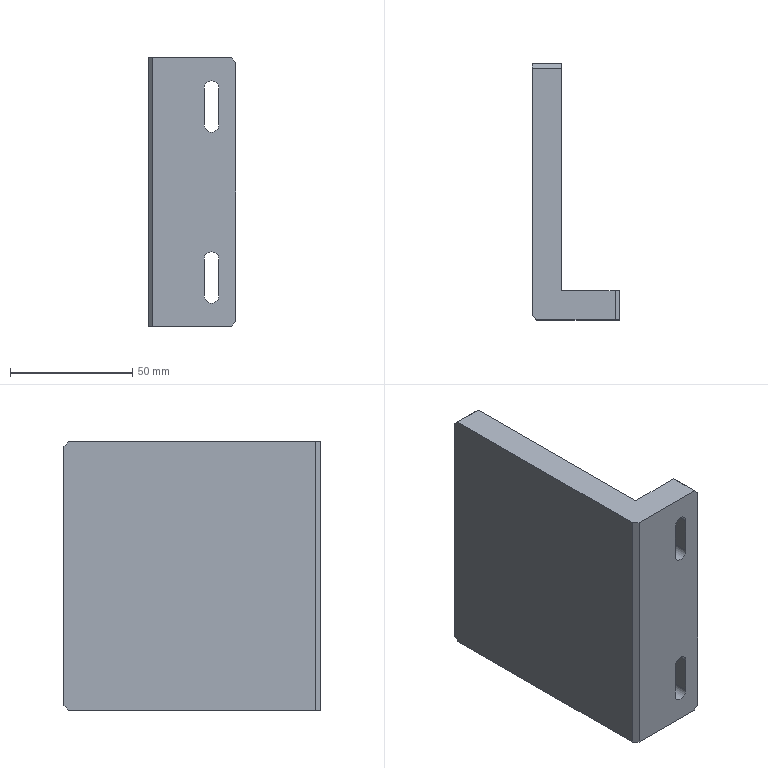Part | SolidWorks | features Chamfer 1, Extrusion 1, HoleWzd 1, ICE 1 | 1 solid | 31 faces | box 36 x 105 x 110 mm | volume 166694 mm3 | plane 17 | cylinder 10 | cone 4 | commonest cylinder face diameters 6 x6 5 x4
STEP:
#1=CARTESIAN_POINT('',(-32.601,41.28,96.5));
#2=VERTEX_POINT('',#1);
#3=CARTESIAN_POINT('',(-32.601,41.28,101.5));
#4=VERTEX_POINT('',#3);
#5=CARTESIAN_POINT('',(-32.601,41.28,99.));
#6=DIRECTION('',(0.,1.,0.));
#7=DIRECTION('',(0.,0.,1.));
#8=AXIS2_PLACEMENT_3D('',#5,#6,#7);
#9=CIRCLE('',#8,2.5);
#10=EDGE_CURVE('',#2,#4,#9,.T.);
#11=ORIENTED_EDGE('',*,*,#10,.F.);
#12=CARTESIAN_POINT('',(-32.601,51.778,96.5));
#13=VERTEX_POINT('',#12);
#14=CARTESIAN_POINT('',(-32.601,51.778,96.5));
#15=DIRECTION('',(0.,1.,0.));
#16=VECTOR('',#15,1000.);
#17=LINE('',#14,#16);
#18=EDGE_CURVE('',#2,#13,#17,.T.);
#19=ORIENTED_EDGE('',*,*,#18,.T.);
#20=CARTESIAN_POINT('',(-32.601,51.778,101.5));
#21=VERTEX_POINT('',#20);
#22=CARTESIAN_POINT('',(-32.601,51.778,99.));
#23=DIRECTION('',(0.,1.,0.));
#24=DIRECTION('',(0.,0.,1.));
#25=AXIS2_PLACEMENT_3D('',#22,#23,#24);
#26=CIRCLE('',#25,2.5);
#27=EDGE_CURVE('',#13,#21,#26,.T.);
#28=ORIENTED_EDGE('',*,*,#27,.T.);
#29=CARTESIAN_POINT('',(-32.601,51.778,101.5));
#30=DIRECTION('',(0.,1.,0.));
#31=VECTOR('',#30,1000.);
#32=LINE('',#29,#31);
#33=EDGE_CURVE('',#4,#21,#32,.T.);
#34=ORIENTED_EDGE('',*,*,#33,.F.);
#35=EDGE_LOOP('',(#11,#19,#28,#34));
#36=FACE_OUTER_BOUND('',#35,.T.);
#37=CARTESIAN_POINT('',(-32.601,51.778,99.));
#38=DIRECTION('',(0.,1.,0.));
#39=DIRECTION('',(0.,0.,1.));
#40=AXIS2_PLACEMENT_3D('',#37,#38,#39);
#41=CYLINDRICAL_SURFACE('',#40,2.5);
#42=ADVANCED_FACE('',(#36),#41,.F.);
#43=CARTESIAN_POINT('',(-32.601,39.778,99.));
#44=VERTEX_POINT('',#43);
#45=CARTESIAN_POINT('',(-32.601,41.28,101.5));
#46=DIRECTION('',(0.,0.515,0.8572));
#47=VECTOR('',#46,1000.);
#48=LINE('',#45,#47);
#49=EDGE_CURVE('',#44,#4,#48,.T.);
#50=ORIENTED_EDGE('',*,*,#49,.F.);
#51=CARTESIAN_POINT('',(-32.601,41.28,96.5));
#52=DIRECTION('',(0.,0.515,-0.8572));
#53=VECTOR('',#52,1000.);
#54=LINE('',#51,#53);
#55=EDGE_CURVE('',#44,#2,#54,.T.);
#56=ORIENTED_EDGE('',*,*,#55,.T.);
#57=ORIENTED_EDGE('',*,*,#10,.T.);
#58=EDGE_LOOP('',(#50,#56,#57));
#59=FACE_OUTER_BOUND('',#58,.T.);
#60=CARTESIAN_POINT('',(-32.601,41.28,99.));
#61=DIRECTION('',(0.,1.,0.));
#62=DIRECTION('',(0.,0.,1.));
#63=AXIS2_PLACEMENT_3D('',#60,#61,#62);
#64=CONICAL_SURFACE('',#63,2.5,1.03);
#65=ADVANCED_FACE('',(#59),#64,.F.);
#66=CARTESIAN_POINT('',(-32.601,41.28,8.5));
#67=VERTEX_POINT('',#66);
#68=CARTESIAN_POINT('',(-32.601,41.28,13.5));
#69=VERTEX_POINT('',#68);
#70=CARTESIAN_POINT('',(-32.601,41.28,11.));
#71=DIRECTION('',(0.,1.,0.));
#72=DIRECTION('',(0.,0.,1.));
#73=AXIS2_PLACEMENT_3D('',#70,#71,#72);
#74=CIRCLE('',#73,2.5);
#75=EDGE_CURVE('',#67,#69,#74,.T.);
#76=ORIENTED_EDGE('',*,*,#75,.F.);
#77=CARTESIAN_POINT('',(-32.601,51.778,8.5));
#78=VERTEX_POINT('',#77);
#79=CARTESIAN_POINT('',(-32.601,51.778,8.5));
#80=DIRECTION('',(0.,1.,0.));
#81=VECTOR('',#80,1000.);
#82=LINE('',#79,#81);
#83=EDGE_CURVE('',#67,#78,#82,.T.);
#84=ORIENTED_EDGE('',*,*,#83,.T.);
#85=CARTESIAN_POINT('',(-32.601,51.778,13.5));
#86=VERTEX_POINT('',#85);
#87=CARTESIAN_POINT('',(-32.601,51.778,11.));
#88=DIRECTION('',(0.,1.,0.));
#89=DIRECTION('',(0.,0.,1.));
#90=AXIS2_PLACEMENT_3D('',#87,#88,#89);
#91=CIRCLE('',#90,2.5);
#92=EDGE_CURVE('',#78,#86,#91,.T.);
#93=ORIENTED_EDGE('',*,*,#92,.T.);
#94=CARTESIAN_POINT('',(-32.601,51.778,13.5));
#95=DIRECTION('',(0.,1.,0.));
#96=VECTOR('',#95,1000.);
#97=LINE('',#94,#96);
#98=EDGE_CURVE('',#69,#86,#97,.T.);
#99=ORIENTED_EDGE('',*,*,#98,.F.);
#100=EDGE_LOOP('',(#76,#84,#93,#99));
#101=FACE_OUTER_BOUND('',#100,.T.);
#102=CARTESIAN_POINT('',(-32.601,51.778,11.));
#103=DIRECTION('',(0.,1.,0.));
#104=DIRECTION('',(0.,0.,1.));
#105=AXIS2_PLACEMENT_3D('',#102,#103,#104);
#106=CYLINDRICAL_SURFACE('',#105,2.5);
#107=ADVANCED_FACE('',(#101),#106,.F.);
#108=CARTESIAN_POINT('',(-32.601,39.778,11.));
#109=VERTEX_POINT('',#108);
#110=CARTESIAN_POINT('',(-32.601,41.28,13.5));
#111=DIRECTION('',(0.,0.515,0.8572));
#112=VECTOR('',#111,1000.);
#113=LINE('',#110,#112);
#114=EDGE_CURVE('',#109,#69,#113,.T.);
#115=ORIENTED_EDGE('',*,*,#114,.F.);
#116=CARTESIAN_POINT('',(-32.601,41.28,8.5));
#117=DIRECTION('',(0.,0.515,-0.8572));
#118=VECTOR('',#117,1000.);
#119=LINE('',#116,#118);
#120=EDGE_CURVE('',#109,#67,#119,.T.);
#121=ORIENTED_EDGE('',*,*,#120,.T.);
#122=ORIENTED_EDGE('',*,*,#75,.T.);
#123=EDGE_LOOP('',(#115,#121,#122));
#124=FACE_OUTER_BOUND('',#123,.T.);
#125=CARTESIAN_POINT('',(-32.601,41.28,11.));
#126=DIRECTION('',(0.,1.,0.));
#127=DIRECTION('',(0.,0.,1.));
#128=AXIS2_PLACEMENT_3D('',#125,#126,#127);
#129=CONICAL_SURFACE('',#128,2.5,1.03);
#130=ADVANCED_FACE('',(#124),#129,.F.);
#131=CARTESIAN_POINT('',(-12.601,-53.222,100.5));
#132=VERTEX_POINT('',#131);
#133=CARTESIAN_POINT('',(-9.601,-53.222,97.5));
#134=VERTEX_POINT('',#133);
#135=CARTESIAN_POINT('',(-12.601,-53.222,97.5));
#136=DIRECTION('',(0.,1.,0.));
#137=DIRECTION('',(0.,0.,1.));
#138=AXIS2_PLACEMENT_3D('',#135,#136,#137);
#139=CIRCLE('',#138,3.);
#140=EDGE_CURVE('',#132,#134,#139,.T.);
#141=ORIENTED_EDGE('',*,*,#140,.F.);
#142=CARTESIAN_POINT('',(-12.601,-41.222,100.5));
#143=VERTEX_POINT('',#142);
#144=CARTESIAN_POINT('',(-12.601,-53.222,100.5));
#145=DIRECTION('',(0.,1.,0.));
#146=VECTOR('',#145,1000.);
#147=LINE('',#144,#146);
#148=EDGE_CURVE('',#132,#143,#147,.T.);
#149=ORIENTED_EDGE('',*,*,#148,.T.);
#150=CARTESIAN_POINT('',(-9.601,-41.222,97.5));
#151=VERTEX_POINT('',#150);
#152=CARTESIAN_POINT('',(-12.601,-41.222,97.5));
#153=DIRECTION('',(0.,1.,0.));
#154=DIRECTION('',(0.,0.,1.));
#155=AXIS2_PLACEMENT_3D('',#152,#153,#154);
#156=CIRCLE('',#155,3.);
#157=EDGE_CURVE('',#143,#151,#156,.T.);
#158=ORIENTED_EDGE('',*,*,#157,.T.);
#159=CARTESIAN_POINT('',(-9.601,-53.222,97.5));
#160=DIRECTION('',(0.,1.,0.));
#161=VECTOR('',#160,1000.);
#162=LINE('',#159,#161);
#163=EDGE_CURVE('',#134,#151,#162,.T.);
#164=ORIENTED_EDGE('',*,*,#163,.F.);
#165=EDGE_LOOP('',(#141,#149,#158,#164));
#166=FACE_OUTER_BOUND('',#165,.T.);
#167=CARTESIAN_POINT('',(-12.601,-53.222,97.5));
#168=DIRECTION('',(0.,1.,0.));
#169=DIRECTION('',(0.,0.,1.));
#170=AXIS2_PLACEMENT_3D('',#167,#168,#169);
#171=CYLINDRICAL_SURFACE('',#170,3.);
#172=ADVANCED_FACE('',(#166),#171,.F.);
#173=CARTESIAN_POINT('',(-12.601,-53.222,30.5));
#174=VERTEX_POINT('',#173);
#175=CARTESIAN_POINT('',(-9.601,-53.222,27.5));
#176=VERTEX_POINT('',#175);
#177=CARTESIAN_POINT('',(-12.601,-53.222,27.5));
#178=DIRECTION('',(0.,1.,0.));
#179=DIRECTION('',(0.,0.,-1.));
#180=AXIS2_PLACEMENT_3D('',#177,#178,#179);
#181=CIRCLE('',#180,3.);
#182=EDGE_CURVE('',#174,#176,#181,.T.);
#183=ORIENTED_EDGE('',*,*,#182,.F.);
#184=CARTESIAN_POINT('',(-12.601,-41.222,30.5));
#185=VERTEX_POINT('',#184);
#186=CARTESIAN_POINT('',(-12.601,-53.222,30.5));
#187=DIRECTION('',(0.,1.,0.));
#188=VECTOR('',#187,1000.);
#189=LINE('',#186,#188);
#190=EDGE_CURVE('',#174,#185,#189,.T.);
#191=ORIENTED_EDGE('',*,*,#190,.T.);
#192=CARTESIAN_POINT('',(-9.601,-41.222,27.5));
#193=VERTEX_POINT('',#192);
#194=CARTESIAN_POINT('',(-12.601,-41.222,27.5));
#195=DIRECTION('',(0.,1.,0.));
#196=DIRECTION('',(0.,0.,-1.));
#197=AXIS2_PLACEMENT_3D('',#194,#195,#196);
#198=CIRCLE('',#197,3.);
#199=EDGE_CURVE('',#185,#193,#198,.T.);
#200=ORIENTED_EDGE('',*,*,#199,.T.);
#201=CARTESIAN_POINT('',(-9.601,-53.222,27.5));
#202=DIRECTION('',(0.,1.,0.));
#203=VECTOR('',#202,1000.);
#204=LINE('',#201,#203);
#205=EDGE_CURVE('',#176,#193,#204,.T.);
#206=ORIENTED_EDGE('',*,*,#205,.F.);
#207=EDGE_LOOP('',(#183,#191,#200,#206));
#208=FACE_OUTER_BOUND('',#207,.T.);
#209=CARTESIAN_POINT('',(-12.601,-53.222,27.5));
#210=DIRECTION('',(0.,1.,0.));
#211=DIRECTION('',(0.,0.,1.));
#212=AXIS2_PLACEMENT_3D('',#209,#210,#211);
#213=CYLINDRICAL_SURFACE('',#212,3.);
#214=ADVANCED_FACE('',(#208),#213,.F.);
#215=CARTESIAN_POINT('',(-32.601,51.778,99.));
#216=DIRECTION('',(0.,1.,0.));
#217=DIRECTION('',(0.,0.,1.));
#218=AXIS2_PLACEMENT_3D('',#215,#216,#217);
#219=CIRCLE('',#218,2.5);
#220=EDGE_CURVE('',#21,#13,#219,.T.);
#221=ORIENTED_EDGE('',*,*,#220,.F.);
#222=ORIENTED_EDGE('',*,*,#27,.F.);
#223=EDGE_LOOP('',(#221,#222));
#224=FACE_BOUND('',#223,.T.);
#225=CARTESIAN_POINT('',(-32.601,51.778,11.));
#226=DIRECTION('',(0.,1.,0.));
#227=DIRECTION('',(0.,0.,1.));
#228=AXIS2_PLACEMENT_3D('',#225,#226,#227);
#229=CIRCLE('',#228,2.5);
#230=EDGE_CURVE('',#86,#78,#229,.T.);
#231=ORIENTED_EDGE('',*,*,#230,.F.);
#232=ORIENTED_EDGE('',*,*,#92,.F.);
#233=EDGE_LOOP('',(#231,#232));
#234=FACE_BOUND('',#233,.T.);
#235=CARTESIAN_POINT('',(-26.601,51.778,108.));
#236=VERTEX_POINT('',#235);
#237=CARTESIAN_POINT('',(-26.601,51.778,2.));
#238=VERTEX_POINT('',#237);
#239=CARTESIAN_POINT('',(-26.601,51.778,110.));
#240=DIRECTION('',(0.,0.,-1.));
#241=VECTOR('',#240,1000.);
#242=LINE('',#239,#241);
#243=EDGE_CURVE('',#236,#238,#242,.T.);
#244=ORIENTED_EDGE('',*,*,#243,.T.);
#245=CARTESIAN_POINT('',(-38.601,51.778,2.));
#246=VERTEX_POINT('',#245);
#247=CARTESIAN_POINT('',(-26.601,51.778,2.));
#248=DIRECTION('',(-1.,0.,0.));
#249=VECTOR('',#248,1000.);
#250=LINE('',#247,#249);
#251=EDGE_CURVE('',#238,#246,#250,.T.);
#252=ORIENTED_EDGE('',*,*,#251,.T.);
#253=CARTESIAN_POINT('',(-38.601,51.778,108.));
#254=VERTEX_POINT('',#253);
#255=CARTESIAN_POINT('',(-38.601,51.778,110.));
#256=DIRECTION('',(0.,0.,-1.));
#257=VECTOR('',#256,1000.);
#258=LINE('',#255,#257);
#259=EDGE_CURVE('',#254,#246,#258,.T.);
#260=ORIENTED_EDGE('',*,*,#259,.F.);
#261=CARTESIAN_POINT('',(-26.601,51.778,108.));
#262=DIRECTION('',(1.,0.,0.));
#263=VECTOR('',#262,1000.);
#264=LINE('',#261,#263);
#265=EDGE_CURVE('',#254,#236,#264,.T.);
#266=ORIENTED_EDGE('',*,*,#265,.T.);
#267=EDGE_LOOP('',(#244,#252,#260,#266));
#268=FACE_OUTER_BOUND('',#267,.T.);
#269=CARTESIAN_POINT('',(-26.601,51.778,110.));
#270=DIRECTION('',(0.,-1.,0.));
#271=DIRECTION('',(1.,0.,0.));
#272=AXIS2_PLACEMENT_3D('',#269,#270,#271);
#273=PLANE('',#272);
#274=ADVANCED_FACE('',(#224,#234,#268),#273,.F.);
#275=CARTESIAN_POINT('',(-38.601,49.778,0.));
#276=VERTEX_POINT('',#275);
#277=CARTESIAN_POINT('',(-38.601,-51.222,0.));
#278=VERTEX_POINT('',#277);
#279=CARTESIAN_POINT('',(-38.601,51.778,0.));
#280=DIRECTION('',(0.,-1.,0.));
#281=VECTOR('',#280,1000.);
#282=LINE('',#279,#281);
#283=EDGE_CURVE('',#276,#278,#282,.T.);
#284=ORIENTED_EDGE('',*,*,#283,.T.);
#285=CARTESIAN_POINT('',(-38.601,-51.222,110.));
#286=VERTEX_POINT('',#285);
#287=CARTESIAN_POINT('',(-38.601,-51.222,110.));
#288=DIRECTION('',(0.,0.,1.));
#289=VECTOR('',#288,1000.);
#290=LINE('',#287,#289);
#291=EDGE_CURVE('',#278,#286,#290,.T.);
#292=ORIENTED_EDGE('',*,*,#291,.T.);
#293=CARTESIAN_POINT('',(-38.601,49.778,110.));
#294=VERTEX_POINT('',#293);
#295=CARTESIAN_POINT('',(-38.601,51.778,110.));
#296=DIRECTION('',(0.,-1.,0.));
#297=VECTOR('',#296,1000.);
#298=LINE('',#295,#297);
#299=EDGE_CURVE('',#294,#286,#298,.T.);
#300=ORIENTED_EDGE('',*,*,#299,.F.);
#301=CARTESIAN_POINT('',(-38.601,49.778,110.));
#302=DIRECTION('',(0.,0.7071,-0.7071));
#303=VECTOR('',#302,1000.);
#304=LINE('',#301,#303);
#305=EDGE_CURVE('',#294,#254,#304,.T.);
#306=ORIENTED_EDGE('',*,*,#305,.T.);
#307=ORIENTED_EDGE('',*,*,#259,.T.);
#308=CARTESIAN_POINT('',(-38.601,51.778,2.));
#309=DIRECTION('',(0.,-0.7071,-0.7071));
#310=VECTOR('',#309,1000.);
#311=LINE('',#308,#310);
#312=EDGE_CURVE('',#246,#276,#311,.T.);
#313=ORIENTED_EDGE('',*,*,#312,.T.);
#314=EDGE_LOOP('',(#284,#292,#300,#306,#307,#313));
#315=FACE_OUTER_BOUND('',#314,.T.);
#316=CARTESIAN_POINT('',(-38.601,51.778,110.));
#317=DIRECTION('',(1.,0.,0.));
#318=DIRECTION('',(0.,1.,0.));
#319=AXIS2_PLACEMENT_3D('',#316,#317,#318);
#320=PLANE('',#319);
#321=ADVANCED_FACE('',(#315),#320,.F.);
#322=CARTESIAN_POINT('',(-15.601,-53.222,82.5));
#323=VERTEX_POINT('',#322);
#324=CARTESIAN_POINT('',(-15.601,-53.222,97.5));
#325=VERTEX_POINT('',#324);
#326=CARTESIAN_POINT('',(-15.601,-53.222,97.5));
#327=DIRECTION('',(0.,0.,1.));
#328=VECTOR('',#327,1000.);
#329=LINE('',#326,#328);
#330=EDGE_CURVE('',#323,#325,#329,.T.);
#331=ORIENTED_EDGE('',*,*,#330,.T.);
#332=CARTESIAN_POINT('',(-12.601,-53.222,97.5));
#333=DIRECTION('',(0.,1.,0.));
#334=DIRECTION('',(0.,0.,1.));
#335=AXIS2_PLACEMENT_3D('',#332,#333,#334);
#336=CIRCLE('',#335,3.);
#337=EDGE_CURVE('',#325,#132,#336,.T.);
#338=ORIENTED_EDGE('',*,*,#337,.T.);
#339=ORIENTED_EDGE('',*,*,#140,.T.);
#340=CARTESIAN_POINT('',(-9.601,-53.222,82.5));
#341=VERTEX_POINT('',#340);
#342=CARTESIAN_POINT('',(-9.601,-53.222,97.5));
#343=DIRECTION('',(0.,0.,-1.));
#344=VECTOR('',#343,1000.);
#345=LINE('',#342,#344);
#346=EDGE_CURVE('',#134,#341,#345,.T.);
#347=ORIENTED_EDGE('',*,*,#346,.T.);
#348=CARTESIAN_POINT('',(-12.601,-53.222,82.5));
#349=DIRECTION('',(0.,1.,0.));
#350=DIRECTION('',(0.,0.,1.));
#351=AXIS2_PLACEMENT_3D('',#348,#349,#350);
#352=CIRCLE('',#351,3.);
#353=EDGE_CURVE('',#341,#323,#352,.T.);
#354=ORIENTED_EDGE('',*,*,#353,.T.);
#355=EDGE_LOOP('',(#331,#338,#339,#347,#354));
#356=FACE_BOUND('',#355,.T.);
#357=CARTESIAN_POINT('',(-9.601,-53.222,12.5));
#358=VERTEX_POINT('',#357);
#359=CARTESIAN_POINT('',(-9.601,-53.222,12.5));
#360=DIRECTION('',(0.,0.,-1.));
#361=VECTOR('',#360,1000.);
#362=LINE('',#359,#361);
#363=EDGE_CURVE('',#176,#358,#362,.T.);
#364=ORIENTED_EDGE('',*,*,#363,.T.);
#365=CARTESIAN_POINT('',(-15.601,-53.222,12.5));
#366=VERTEX_POINT('',#365);
#367=CARTESIAN_POINT('',(-12.601,-53.222,12.5));
#368=DIRECTION('',(0.,1.,0.));
#369=DIRECTION('',(0.,0.,-1.));
#370=AXIS2_PLACEMENT_3D('',#367,#368,#369);
#371=CIRCLE('',#370,3.);
#372=EDGE_CURVE('',#358,#366,#371,.T.);
#373=ORIENTED_EDGE('',*,*,#372,.T.);
#374=CARTESIAN_POINT('',(-15.601,-53.222,27.5));
#375=VERTEX_POINT('',#374);
#376=CARTESIAN_POINT('',(-15.601,-53.222,12.5));
#377=DIRECTION('',(0.,0.,1.));
#378=VECTOR('',#377,1000.);
#379=LINE('',#376,#378);
#380=EDGE_CURVE('',#366,#375,#379,.T.);
#381=ORIENTED_EDGE('',*,*,#380,.T.);
#382=CARTESIAN_POINT('',(-12.601,-53.222,27.5));
#383=DIRECTION('',(0.,1.,0.));
#384=DIRECTION('',(0.,0.,-1.));
#385=AXIS2_PLACEMENT_3D('',#382,#383,#384);
#386=CIRCLE('',#385,3.);
#387=EDGE_CURVE('',#375,#174,#386,.T.);
#388=ORIENTED_EDGE('',*,*,#387,.T.);
#389=ORIENTED_EDGE('',*,*,#182,.T.);
#390=EDGE_LOOP('',(#364,#373,#381,#388,#389));
#391=FACE_BOUND('',#390,.T.);
#392=CARTESIAN_POINT('',(-36.601,-53.222,110.));
#393=VERTEX_POINT('',#392);
#394=CARTESIAN_POINT('',(-4.601,-53.222,110.));
#395=VERTEX_POINT('',#394);
#396=CARTESIAN_POINT('',(-38.601,-53.222,110.));
#397=DIRECTION('',(1.,0.,0.));
#398=VECTOR('',#397,1000.);
#399=LINE('',#396,#398);
#400=EDGE_CURVE('',#393,#395,#399,.T.);
#401=ORIENTED_EDGE('',*,*,#400,.F.);
#402=CARTESIAN_POINT('',(-36.601,-53.222,0.));
#403=VERTEX_POINT('',#402);
#404=CARTESIAN_POINT('',(-36.601,-53.222,110.));
#405=DIRECTION('',(0.,0.,-1.));
#406=VECTOR('',#405,1000.);
#407=LINE('',#404,#406);
#408=EDGE_CURVE('',#393,#403,#407,.T.);
#409=ORIENTED_EDGE('',*,*,#408,.T.);
#410=CARTESIAN_POINT('',(-4.601,-53.222,0.));
#411=VERTEX_POINT('',#410);
#412=CARTESIAN_POINT('',(-38.601,-53.222,0.));
#413=DIRECTION('',(1.,0.,0.));
#414=VECTOR('',#413,1000.);
#415=LINE('',#412,#414);
#416=EDGE_CURVE('',#403,#411,#415,.T.);
#417=ORIENTED_EDGE('',*,*,#416,.T.);
#418=CARTESIAN_POINT('',(-2.601,-53.222,2.));
#419=VERTEX_POINT('',#418);
#420=CARTESIAN_POINT('',(-2.601,-53.222,2.));
#421=DIRECTION('',(0.7071,0.,0.7071));
#422=VECTOR('',#421,1000.);
#423=LINE('',#420,#422);
#424=EDGE_CURVE('',#411,#419,#423,.T.);
#425=ORIENTED_EDGE('',*,*,#424,.T.);
#426=CARTESIAN_POINT('',(-2.601,-53.222,108.));
#427=VERTEX_POINT('',#426);
#428=CARTESIAN_POINT('',(-2.601,-53.222,110.));
#429=DIRECTION('',(0.,0.,-1.));
#430=VECTOR('',#429,1000.);
#431=LINE('',#428,#430);
#432=EDGE_CURVE('',#427,#419,#431,.T.);
#433=ORIENTED_EDGE('',*,*,#432,.F.);
#434=CARTESIAN_POINT('',(-4.601,-53.222,110.));
#435=DIRECTION('',(-0.7071,0.,0.7071));
#436=VECTOR('',#435,1000.);
#437=LINE('',#434,#436);
#438=EDGE_CURVE('',#427,#395,#437,.T.);
#439=ORIENTED_EDGE('',*,*,#438,.T.);
#440=EDGE_LOOP('',(#401,#409,#417,#425,#433,#439));
#441=FACE_OUTER_BOUND('',#440,.T.);
#442=CARTESIAN_POINT('',(-38.601,-53.222,110.));
#443=DIRECTION('',(0.,1.,0.));
#444=DIRECTION('',(0.,0.,1.));
#445=AXIS2_PLACEMENT_3D('',#442,#443,#444);
#446=PLANE('',#445);
#447=ADVANCED_FACE('',(#356,#391,#441),#446,.F.);
#448=ORIENTED_EDGE('',*,*,#432,.T.);
#449=CARTESIAN_POINT('',(-2.601,-41.222,2.));
#450=VERTEX_POINT('',#449);
#451=CARTESIAN_POINT('',(-2.601,-53.222,2.));
#452=DIRECTION('',(0.,1.,0.));
#453=VECTOR('',#452,1000.);
#454=LINE('',#451,#453);
#455=EDGE_CURVE('',#419,#450,#454,.T.);
#456=ORIENTED_EDGE('',*,*,#455,.T.);
#457=CARTESIAN_POINT('',(-2.601,-41.222,108.));
#458=VERTEX_POINT('',#457);
#459=CARTESIAN_POINT('',(-2.601,-41.222,110.));
#460=DIRECTION('',(0.,0.,-1.));
#461=VECTOR('',#460,1000.);
#462=LINE('',#459,#461);
#463=EDGE_CURVE('',#458,#450,#462,.T.);
#464=ORIENTED_EDGE('',*,*,#463,.F.);
#465=CARTESIAN_POINT('',(-2.601,-53.222,108.));
#466=DIRECTION('',(0.,-1.,0.));
#467=VECTOR('',#466,1000.);
#468=LINE('',#465,#467);
#469=EDGE_CURVE('',#458,#427,#468,.T.);
#470=ORIENTED_EDGE('',*,*,#469,.T.);
#471=EDGE_LOOP('',(#448,#456,#464,#470));
#472=FACE_OUTER_BOUND('',#471,.T.);
#473=CARTESIAN_POINT('',(-2.601,-53.222,110.));
#474=DIRECTION('',(-1.,0.,0.));
#475=DIRECTION('',(0.,0.,1.));
#476=AXIS2_PLACEMENT_3D('',#473,#474,#475);
#477=PLANE('',#476);
#478=ADVANCED_FACE('',(#472),#477,.F.);
#479=CARTESIAN_POINT('',(-9.601,-41.222,82.5));
#480=VERTEX_POINT('',#479);
#481=CARTESIAN_POINT('',(-9.601,-41.222,97.5));
#482=DIRECTION('',(0.,0.,-1.));
#483=VECTOR('',#482,1000.);
#484=LINE('',#481,#483);
#485=EDGE_CURVE('',#151,#480,#484,.T.);
#486=ORIENTED_EDGE('',*,*,#485,.F.);
#487=ORIENTED_EDGE('',*,*,#157,.F.);
#488=CARTESIAN_POINT('',(-15.601,-41.222,97.5));
#489=VERTEX_POINT('',#488);
#490=CARTESIAN_POINT('',(-12.601,-41.222,97.5));
#491=DIRECTION('',(0.,1.,0.));
#492=DIRECTION('',(0.,0.,1.));
#493=AXIS2_PLACEMENT_3D('',#490,#491,#492);
#494=CIRCLE('',#493,3.);
#495=EDGE_CURVE('',#489,#143,#494,.T.);
#496=ORIENTED_EDGE('',*,*,#495,.F.);
#497=CARTESIAN_POINT('',(-15.601,-41.222,82.5));
#498=VERTEX_POINT('',#497);
#499=CARTESIAN_POINT('',(-15.601,-41.222,97.5));
#500=DIRECTION('',(0.,0.,1.));
#501=VECTOR('',#500,1000.);
#502=LINE('',#499,#501);
#503=EDGE_CURVE('',#498,#489,#502,.T.);
#504=ORIENTED_EDGE('',*,*,#503,.F.);
#505=CARTESIAN_POINT('',(-12.601,-41.222,82.5));
#506=DIRECTION('',(0.,1.,0.));
#507=DIRECTION('',(0.,0.,1.));
#508=AXIS2_PLACEMENT_3D('',#505,#506,#507);
#509=CIRCLE('',#508,3.);
#510=EDGE_CURVE('',#480,#498,#509,.T.);
#511=ORIENTED_EDGE('',*,*,#510,.F.);
#512=EDGE_LOOP('',(#486,#487,#496,#504,#511));
#513=FACE_BOUND('',#512,.T.);
#514=CARTESIAN_POINT('',(-15.601,-41.222,12.5));
#515=VERTEX_POINT('',#514);
#516=CARTESIAN_POINT('',(-15.601,-41.222,27.5));
#517=VERTEX_POINT('',#516);
#518=CARTESIAN_POINT('',(-15.601,-41.222,12.5));
#519=DIRECTION('',(0.,0.,1.));
#520=VECTOR('',#519,1000.);
#521=LINE('',#518,#520);
#522=EDGE_CURVE('',#515,#517,#521,.T.);
#523=ORIENTED_EDGE('',*,*,#522,.F.);
#524=CARTESIAN_POINT('',(-9.601,-41.222,12.5));
#525=VERTEX_POINT('',#524);
#526=CARTESIAN_POINT('',(-12.601,-41.222,12.5));
#527=DIRECTION('',(0.,1.,0.));
#528=DIRECTION('',(0.,0.,-1.));
#529=AXIS2_PLACEMENT_3D('',#526,#527,#528);
#530=CIRCLE('',#529,3.);
#531=EDGE_CURVE('',#525,#515,#530,.T.);
#532=ORIENTED_EDGE('',*,*,#531,.F.);
#533=CARTESIAN_POINT('',(-9.601,-41.222,12.5));
#534=DIRECTION('',(0.,0.,-1.));
#535=VECTOR('',#534,1000.);
#536=LINE('',#533,#535);
#537=EDGE_CURVE('',#193,#525,#536,.T.);
#538=ORIENTED_EDGE('',*,*,#537,.F.);
#539=ORIENTED_EDGE('',*,*,#199,.F.);
#540=CARTESIAN_POINT('',(-12.601,-41.222,27.5));
#541=DIRECTION('',(0.,1.,0.));
#542=DIRECTION('',(0.,0.,-1.));
#543=AXIS2_PLACEMENT_3D('',#540,#541,#542);
#544=CIRCLE('',#543,3.);
#545=EDGE_CURVE('',#517,#185,#544,.T.);
#546=ORIENTED_EDGE('',*,*,#545,.F.);
#547=EDGE_LOOP('',(#523,#532,#538,#539,#546));
#548=FACE_BOUND('',#547,.T.);
#549=ORIENTED_EDGE('',*,*,#463,.T.);
#550=CARTESIAN_POINT('',(-4.601,-41.222,0.));
#551=VERTEX_POINT('',#550);
#552=CARTESIAN_POINT('',(-2.601,-41.222,2.));
#553=DIRECTION('',(-0.7071,0.,-0.7071));
#554=VECTOR('',#553,1000.);
#555=LINE('',#552,#554);
#556=EDGE_CURVE('',#450,#551,#555,.T.);
#557=ORIENTED_EDGE('',*,*,#556,.T.);
#558=CARTESIAN_POINT('',(-26.601,-41.222,0.));
#559=VERTEX_POINT('',#558);
#560=CARTESIAN_POINT('',(-2.601,-41.222,0.));
#561=DIRECTION('',(-1.,0.,0.));
#562=VECTOR('',#561,1000.);
#563=LINE('',#560,#562);
#564=EDGE_CURVE('',#551,#559,#563,.T.);
#565=ORIENTED_EDGE('',*,*,#564,.T.);
#566=CARTESIAN_POINT('',(-26.601,-41.222,110.));
#567=VERTEX_POINT('',#566);
#568=CARTESIAN_POINT('',(-26.601,-41.222,110.));
#569=DIRECTION('',(0.,0.,-1.));
#570=VECTOR('',#569,1000.);
#571=LINE('',#568,#570);
#572=EDGE_CURVE('',#567,#559,#571,.T.);
#573=ORIENTED_EDGE('',*,*,#572,.F.);
#574=CARTESIAN_POINT('',(-4.601,-41.222,110.));
#575=VERTEX_POINT('',#574);
#576=CARTESIAN_POINT('',(-2.601,-41.222,110.));
#577=DIRECTION('',(-1.,0.,0.));
#578=VECTOR('',#577,1000.);
#579=LINE('',#576,#578);
#580=EDGE_CURVE('',#575,#567,#579,.T.);
#581=ORIENTED_EDGE('',*,*,#580,.F.);
#582=CARTESIAN_POINT('',(-4.601,-41.222,110.));
#583=DIRECTION('',(0.7071,0.,-0.7071));
#584=VECTOR('',#583,1000.);
#585=LINE('',#582,#584);
#586=EDGE_CURVE('',#575,#458,#585,.T.);
#587=ORIENTED_EDGE('',*,*,#586,.T.);
#588=EDGE_LOOP('',(#549,#557,#565,#573,#581,#587));
#589=FACE_OUTER_BOUND('',#588,.T.);
#590=CARTESIAN_POINT('',(-2.601,-41.222,110.));
#591=DIRECTION('',(0.,-1.,0.));
#592=DIRECTION('',(0.,0.,-1.));
#593=AXIS2_PLACEMENT_3D('',#590,#591,#592);
#594=PLANE('',#593);
#595=ADVANCED_FACE('',(#513,#548,#589),#594,.F.);
#596=CARTESIAN_POINT('',(-26.601,49.778,0.));
#597=VERTEX_POINT('',#596);
#598=CARTESIAN_POINT('',(-26.601,-41.222,0.));
#599=DIRECTION('',(0.,1.,0.));
#600=VECTOR('',#599,1000.);
#601=LINE('',#598,#600);
#602=EDGE_CURVE('',#559,#597,#601,.T.);
#603=ORIENTED_EDGE('',*,*,#602,.T.);
#604=CARTESIAN_POINT('',(-26.601,51.778,2.));
#605=DIRECTION('',(0.,0.7071,0.7071));
#606=VECTOR('',#605,1000.);
#607=LINE('',#604,#606);
#608=EDGE_CURVE('',#597,#238,#607,.T.);
#609=ORIENTED_EDGE('',*,*,#608,.T.);
#610=ORIENTED_EDGE('',*,*,#243,.F.);
#611=CARTESIAN_POINT('',(-26.601,49.778,110.));
#612=VERTEX_POINT('',#611);
#613=CARTESIAN_POINT('',(-26.601,49.778,110.));
#614=DIRECTION('',(0.,-0.7071,0.7071));
#615=VECTOR('',#614,1000.);
#616=LINE('',#613,#615);
#617=EDGE_CURVE('',#236,#612,#616,.T.);
#618=ORIENTED_EDGE('',*,*,#617,.T.);
#619=CARTESIAN_POINT('',(-26.601,-41.222,110.));
#620=DIRECTION('',(0.,1.,0.));
#621=VECTOR('',#620,1000.);
#622=LINE('',#619,#621);
#623=EDGE_CURVE('',#567,#612,#622,.T.);
#624=ORIENTED_EDGE('',*,*,#623,.F.);
#625=ORIENTED_EDGE('',*,*,#572,.T.);
#626=EDGE_LOOP('',(#603,#609,#610,#618,#624,#625));
#627=FACE_OUTER_BOUND('',#626,.T.);
#628=CARTESIAN_POINT('',(-26.601,-41.222,110.));
#629=DIRECTION('',(-1.,0.,0.));
#630=DIRECTION('',(0.,0.,1.));
#631=AXIS2_PLACEMENT_3D('',#628,#629,#630);
#632=PLANE('',#631);
#633=ADVANCED_FACE('',(#627),#632,.F.);
#634=ORIENTED_EDGE('',*,*,#299,.T.);
#635=CARTESIAN_POINT('',(-44.912,-44.912,110.));
#636=DIRECTION('',(0.7071,-0.7071,0.));
#637=VECTOR('',#636,1000.);
#638=LINE('',#635,#637);
#639=EDGE_CURVE('',#286,#393,#638,.T.);
#640=ORIENTED_EDGE('',*,*,#639,.T.);
#641=ORIENTED_EDGE('',*,*,#400,.T.);
#642=CARTESIAN_POINT('',(-4.601,-41.222,110.));
#643=DIRECTION('',(0.,1.,0.));
#644=VECTOR('',#643,1000.);
#645=LINE('',#642,#644);
#646=EDGE_CURVE('',#395,#575,#645,.T.);
#647=ORIENTED_EDGE('',*,*,#646,.T.);
#648=ORIENTED_EDGE('',*,*,#580,.T.);
#649=ORIENTED_EDGE('',*,*,#623,.T.);
#650=CARTESIAN_POINT('',(-38.601,49.778,110.));
#651=DIRECTION('',(-1.,0.,0.));
#652=VECTOR('',#651,1000.);
#653=LINE('',#650,#652);
#654=EDGE_CURVE('',#612,#294,#653,.T.);
#655=ORIENTED_EDGE('',*,*,#654,.T.);
#656=EDGE_LOOP('',(#634,#640,#641,#647,#648,#649,#655));
#657=FACE_OUTER_BOUND('',#656,.T.);
#658=CARTESIAN_POINT('',(0.,0.,110.));
#659=DIRECTION('',(0.,0.,1.));
#660=DIRECTION('',(1.,0.,0.));
#661=AXIS2_PLACEMENT_3D('',#658,#659,#660);
#662=PLANE('',#661);
#663=ADVANCED_FACE('',(#657),#662,.T.);
#664=ORIENTED_EDGE('',*,*,#416,.F.);
#665=CARTESIAN_POINT('',(-36.601,-53.222,0.));
#666=DIRECTION('',(-0.7071,0.7071,0.));
#667=VECTOR('',#666,1000.);
#668=LINE('',#665,#667);
#669=EDGE_CURVE('',#403,#278,#668,.T.);
#670=ORIENTED_EDGE('',*,*,#669,.T.);
#671=ORIENTED_EDGE('',*,*,#283,.F.);
#672=CARTESIAN_POINT('',(0.,49.778,0.));
#673=DIRECTION('',(1.,0.,0.));
#674=VECTOR('',#673,1000.);
#675=LINE('',#672,#674);
#676=EDGE_CURVE('',#276,#597,#675,.T.);
#677=ORIENTED_EDGE('',*,*,#676,.T.);
#678=ORIENTED_EDGE('',*,*,#602,.F.);
#679=ORIENTED_EDGE('',*,*,#564,.F.);
#680=CARTESIAN_POINT('',(-4.601,0.,0.));
#681=DIRECTION('',(0.,-1.,0.));
#682=VECTOR('',#681,1000.);
#683=LINE('',#680,#682);
#684=EDGE_CURVE('',#551,#411,#683,.T.);
#685=ORIENTED_EDGE('',*,*,#684,.T.);
#686=EDGE_LOOP('',(#664,#670,#671,#677,#678,#679,#685));
#687=FACE_OUTER_BOUND('',#686,.T.);
#688=CARTESIAN_POINT('',(0.,0.,0.));
#689=DIRECTION('',(0.,0.,1.));
#690=DIRECTION('',(1.,0.,0.));
#691=AXIS2_PLACEMENT_3D('',#688,#689,#690);
#692=PLANE('',#691);
#693=ADVANCED_FACE('',(#687),#692,.F.);
#694=ORIENTED_EDGE('',*,*,#639,.F.);
#695=ORIENTED_EDGE('',*,*,#291,.F.);
#696=ORIENTED_EDGE('',*,*,#669,.F.);
#697=ORIENTED_EDGE('',*,*,#408,.F.);
#698=EDGE_LOOP('',(#694,#695,#696,#697));
#699=FACE_OUTER_BOUND('',#698,.T.);
#700=CARTESIAN_POINT('',(-36.601,-53.222,110.));
#701=DIRECTION('',(0.7071,0.7071,0.));
#702=DIRECTION('',(0.,0.,-1.));
#703=AXIS2_PLACEMENT_3D('',#700,#701,#702);
#704=PLANE('',#703);
#705=ADVANCED_FACE('',(#699),#704,.F.);
#706=ORIENTED_EDGE('',*,*,#424,.F.);
#707=ORIENTED_EDGE('',*,*,#684,.F.);
#708=ORIENTED_EDGE('',*,*,#556,.F.);
#709=ORIENTED_EDGE('',*,*,#455,.F.);
#710=EDGE_LOOP('',(#706,#707,#708,#709));
#711=FACE_OUTER_BOUND('',#710,.T.);
#712=CARTESIAN_POINT('',(-2.601,-53.222,2.));
#713=DIRECTION('',(-0.7071,0.,0.7071));
#714=DIRECTION('',(0.,1.,0.));
#715=AXIS2_PLACEMENT_3D('',#712,#713,#714);
#716=PLANE('',#715);
#717=ADVANCED_FACE('',(#711),#716,.F.);
#718=ORIENTED_EDGE('',*,*,#438,.F.);
#719=ORIENTED_EDGE('',*,*,#469,.F.);
#720=ORIENTED_EDGE('',*,*,#586,.F.);
#721=ORIENTED_EDGE('',*,*,#646,.F.);
#722=EDGE_LOOP('',(#718,#719,#720,#721));
#723=FACE_OUTER_BOUND('',#722,.T.);
#724=CARTESIAN_POINT('',(-4.601,0.,110.));
#725=DIRECTION('',(0.7071,0.,0.7071));
#726=DIRECTION('',(0.,-1.,0.));
#727=AXIS2_PLACEMENT_3D('',#724,#725,#726);
#728=PLANE('',#727);
#729=ADVANCED_FACE('',(#723),#728,.T.);
#730=ORIENTED_EDGE('',*,*,#608,.F.);
#731=ORIENTED_EDGE('',*,*,#676,.F.);
#732=ORIENTED_EDGE('',*,*,#312,.F.);
#733=ORIENTED_EDGE('',*,*,#251,.F.);
#734=EDGE_LOOP('',(#730,#731,#732,#733));
#735=FACE_OUTER_BOUND('',#734,.T.);
#736=CARTESIAN_POINT('',(-26.601,51.778,2.));
#737=DIRECTION('',(0.,-0.7071,0.7071));
#738=DIRECTION('',(-1.,0.,0.));
#739=AXIS2_PLACEMENT_3D('',#736,#737,#738);
#740=PLANE('',#739);
#741=ADVANCED_FACE('',(#735),#740,.F.);
#742=ORIENTED_EDGE('',*,*,#617,.F.);
#743=ORIENTED_EDGE('',*,*,#265,.F.);
#744=ORIENTED_EDGE('',*,*,#305,.F.);
#745=ORIENTED_EDGE('',*,*,#654,.F.);
#746=EDGE_LOOP('',(#742,#743,#744,#745));
#747=FACE_OUTER_BOUND('',#746,.T.);
#748=CARTESIAN_POINT('',(0.,49.778,110.));
#749=DIRECTION('',(0.,0.7071,0.7071));
#750=DIRECTION('',(1.,0.,0.));
#751=AXIS2_PLACEMENT_3D('',#748,#749,#750);
#752=PLANE('',#751);
#753=ADVANCED_FACE('',(#747),#752,.T.);
#754=ORIENTED_EDGE('',*,*,#531,.T.);
#755=CARTESIAN_POINT('',(-15.601,-53.222,12.5));
#756=DIRECTION('',(0.,1.,0.));
#757=VECTOR('',#756,1000.);
#758=LINE('',#755,#757);
#759=EDGE_CURVE('',#366,#515,#758,.T.);
#760=ORIENTED_EDGE('',*,*,#759,.F.);
#761=ORIENTED_EDGE('',*,*,#372,.F.);
#762=CARTESIAN_POINT('',(-9.601,-53.222,12.5));
#763=DIRECTION('',(0.,1.,0.));
#764=VECTOR('',#763,1000.);
#765=LINE('',#762,#764);
#766=EDGE_CURVE('',#358,#525,#765,.T.);
#767=ORIENTED_EDGE('',*,*,#766,.T.);
#768=EDGE_LOOP('',(#754,#760,#761,#767));
#769=FACE_OUTER_BOUND('',#768,.T.);
#770=CARTESIAN_POINT('',(-12.601,-53.222,12.5));
#771=DIRECTION('',(0.,1.,0.));
#772=DIRECTION('',(0.,0.,1.));
#773=AXIS2_PLACEMENT_3D('',#770,#771,#772);
#774=CYLINDRICAL_SURFACE('',#773,3.);
#775=ADVANCED_FACE('',(#769),#774,.F.);
#776=ORIENTED_EDGE('',*,*,#537,.T.);
#777=ORIENTED_EDGE('',*,*,#766,.F.);
#778=ORIENTED_EDGE('',*,*,#363,.F.);
#779=ORIENTED_EDGE('',*,*,#205,.T.);
#780=EDGE_LOOP('',(#776,#777,#778,#779));
#781=FACE_OUTER_BOUND('',#780,.T.);
#782=CARTESIAN_POINT('',(-9.601,-53.222,12.5));
#783=DIRECTION('',(1.,0.,0.));
#784=DIRECTION('',(0.,0.,-1.));
#785=AXIS2_PLACEMENT_3D('',#782,#783,#784);
#786=PLANE('',#785);
#787=ADVANCED_FACE('',(#781),#786,.F.);
#788=ORIENTED_EDGE('',*,*,#190,.F.);
#789=ORIENTED_EDGE('',*,*,#387,.F.);
#790=CARTESIAN_POINT('',(-15.601,-53.222,27.5));
#791=DIRECTION('',(0.,1.,0.));
#792=VECTOR('',#791,1000.);
#793=LINE('',#790,#792);
#794=EDGE_CURVE('',#375,#517,#793,.T.);
#795=ORIENTED_EDGE('',*,*,#794,.T.);
#796=ORIENTED_EDGE('',*,*,#545,.T.);
#797=EDGE_LOOP('',(#788,#789,#795,#796));
#798=FACE_OUTER_BOUND('',#797,.T.);
#799=CARTESIAN_POINT('',(-12.601,-53.222,27.5));
#800=DIRECTION('',(0.,1.,0.));
#801=DIRECTION('',(0.,0.,1.));
#802=AXIS2_PLACEMENT_3D('',#799,#800,#801);
#803=CYLINDRICAL_SURFACE('',#802,3.);
#804=ADVANCED_FACE('',(#798),#803,.F.);
#805=ORIENTED_EDGE('',*,*,#522,.T.);
#806=ORIENTED_EDGE('',*,*,#794,.F.);
#807=ORIENTED_EDGE('',*,*,#380,.F.);
#808=ORIENTED_EDGE('',*,*,#759,.T.);
#809=EDGE_LOOP('',(#805,#806,#807,#808));
#810=FACE_OUTER_BOUND('',#809,.T.);
#811=CARTESIAN_POINT('',(-15.601,-53.222,12.5));
#812=DIRECTION('',(-1.,0.,0.));
#813=DIRECTION('',(0.,0.,1.));
#814=AXIS2_PLACEMENT_3D('',#811,#812,#813);
#815=PLANE('',#814);
#816=ADVANCED_FACE('',(#810),#815,.F.);
#817=ORIENTED_EDGE('',*,*,#148,.F.);
#818=ORIENTED_EDGE('',*,*,#337,.F.);
#819=CARTESIAN_POINT('',(-15.601,-53.222,97.5));
#820=DIRECTION('',(0.,1.,0.));
#821=VECTOR('',#820,1000.);
#822=LINE('',#819,#821);
#823=EDGE_CURVE('',#325,#489,#822,.T.);
#824=ORIENTED_EDGE('',*,*,#823,.T.);
#825=ORIENTED_EDGE('',*,*,#495,.T.);
#826=EDGE_LOOP('',(#817,#818,#824,#825));
#827=FACE_OUTER_BOUND('',#826,.T.);
#828=CARTESIAN_POINT('',(-12.601,-53.222,97.5));
#829=DIRECTION('',(0.,1.,0.));
#830=DIRECTION('',(0.,0.,1.));
#831=AXIS2_PLACEMENT_3D('',#828,#829,#830);
#832=CYLINDRICAL_SURFACE('',#831,3.);
#833=ADVANCED_FACE('',(#827),#832,.F.);
#834=ORIENTED_EDGE('',*,*,#503,.T.);
#835=ORIENTED_EDGE('',*,*,#823,.F.);
#836=ORIENTED_EDGE('',*,*,#330,.F.);
#837=CARTESIAN_POINT('',(-15.601,-53.222,82.5));
#838=DIRECTION('',(0.,1.,0.));
#839=VECTOR('',#838,1000.);
#840=LINE('',#837,#839);
#841=EDGE_CURVE('',#323,#498,#840,.T.);
#842=ORIENTED_EDGE('',*,*,#841,.T.);
#843=EDGE_LOOP('',(#834,#835,#836,#842));
#844=FACE_OUTER_BOUND('',#843,.T.);
#845=CARTESIAN_POINT('',(-15.601,-53.222,97.5));
#846=DIRECTION('',(-1.,0.,0.));
#847=DIRECTION('',(0.,0.,1.));
#848=AXIS2_PLACEMENT_3D('',#845,#846,#847);
#849=PLANE('',#848);
#850=ADVANCED_FACE('',(#844),#849,.F.);
#851=ORIENTED_EDGE('',*,*,#510,.T.);
#852=ORIENTED_EDGE('',*,*,#841,.F.);
#853=ORIENTED_EDGE('',*,*,#353,.F.);
#854=CARTESIAN_POINT('',(-9.601,-53.222,82.5));
#855=DIRECTION('',(0.,1.,0.));
#856=VECTOR('',#855,1000.);
#857=LINE('',#854,#856);
#858=EDGE_CURVE('',#341,#480,#857,.T.);
#859=ORIENTED_EDGE('',*,*,#858,.T.);
#860=EDGE_LOOP('',(#851,#852,#853,#859));
#861=FACE_OUTER_BOUND('',#860,.T.);
#862=CARTESIAN_POINT('',(-12.601,-53.222,82.5));
#863=DIRECTION('',(0.,1.,0.));
#864=DIRECTION('',(0.,0.,1.));
#865=AXIS2_PLACEMENT_3D('',#862,#863,#864);
#866=CYLINDRICAL_SURFACE('',#865,3.);
#867=ADVANCED_FACE('',(#861),#866,.F.);
#868=ORIENTED_EDGE('',*,*,#485,.T.);
#869=ORIENTED_EDGE('',*,*,#858,.F.);
#870=ORIENTED_EDGE('',*,*,#346,.F.);
#871=ORIENTED_EDGE('',*,*,#163,.T.);
#872=EDGE_LOOP('',(#868,#869,#870,#871));
#873=FACE_OUTER_BOUND('',#872,.T.);
#874=CARTESIAN_POINT('',(-9.601,-53.222,97.5));
#875=DIRECTION('',(1.,0.,0.));
#876=DIRECTION('',(0.,0.,-1.));
#877=AXIS2_PLACEMENT_3D('',#874,#875,#876);
#878=PLANE('',#877);
#879=ADVANCED_FACE('',(#873),#878,.F.);
#880=ORIENTED_EDGE('',*,*,#120,.F.);
#881=ORIENTED_EDGE('',*,*,#114,.T.);
#882=CARTESIAN_POINT('',(-32.601,41.28,11.));
#883=DIRECTION('',(0.,1.,0.));
#884=DIRECTION('',(0.,0.,1.));
#885=AXIS2_PLACEMENT_3D('',#882,#883,#884);
#886=CIRCLE('',#885,2.5);
#887=EDGE_CURVE('',#69,#67,#886,.T.);
#888=ORIENTED_EDGE('',*,*,#887,.T.);
#889=EDGE_LOOP('',(#880,#881,#888));
#890=FACE_OUTER_BOUND('',#889,.T.);
#891=CARTESIAN_POINT('',(-32.601,41.28,11.));
#892=DIRECTION('',(0.,1.,0.));
#893=DIRECTION('',(0.,0.,1.));
#894=AXIS2_PLACEMENT_3D('',#891,#892,#893);
#895=CONICAL_SURFACE('',#894,2.5,1.03);
#896=ADVANCED_FACE('',(#890),#895,.F.);
#897=ORIENTED_EDGE('',*,*,#83,.F.);
#898=ORIENTED_EDGE('',*,*,#887,.F.);
#899=ORIENTED_EDGE('',*,*,#98,.T.);
#900=ORIENTED_EDGE('',*,*,#230,.T.);
#901=EDGE_LOOP('',(#897,#898,#899,#900));
#902=FACE_OUTER_BOUND('',#901,.T.);
#903=CARTESIAN_POINT('',(-32.601,51.778,11.));
#904=DIRECTION('',(0.,1.,0.));
#905=DIRECTION('',(0.,0.,1.));
#906=AXIS2_PLACEMENT_3D('',#903,#904,#905);
#907=CYLINDRICAL_SURFACE('',#906,2.5);
#908=ADVANCED_FACE('',(#902),#907,.F.);
#909=ORIENTED_EDGE('',*,*,#55,.F.);
#910=ORIENTED_EDGE('',*,*,#49,.T.);
#911=CARTESIAN_POINT('',(-32.601,41.28,99.));
#912=DIRECTION('',(0.,1.,0.));
#913=DIRECTION('',(0.,0.,1.));
#914=AXIS2_PLACEMENT_3D('',#911,#912,#913);
#915=CIRCLE('',#914,2.5);
#916=EDGE_CURVE('',#4,#2,#915,.T.);
#917=ORIENTED_EDGE('',*,*,#916,.T.);
#918=EDGE_LOOP('',(#909,#910,#917));
#919=FACE_OUTER_BOUND('',#918,.T.);
#920=CARTESIAN_POINT('',(-32.601,41.28,99.));
#921=DIRECTION('',(0.,1.,0.));
#922=DIRECTION('',(0.,0.,1.));
#923=AXIS2_PLACEMENT_3D('',#920,#921,#922);
#924=CONICAL_SURFACE('',#923,2.5,1.03);
#925=ADVANCED_FACE('',(#919),#924,.F.);
#926=ORIENTED_EDGE('',*,*,#18,.F.);
#927=ORIENTED_EDGE('',*,*,#916,.F.);
#928=ORIENTED_EDGE('',*,*,#33,.T.);
#929=ORIENTED_EDGE('',*,*,#220,.T.);
#930=EDGE_LOOP('',(#926,#927,#928,#929));
#931=FACE_OUTER_BOUND('',#930,.T.);
#932=CARTESIAN_POINT('',(-32.601,51.778,99.));
#933=DIRECTION('',(0.,1.,0.));
#934=DIRECTION('',(0.,0.,1.));
#935=AXIS2_PLACEMENT_3D('',#932,#933,#934);
#936=CYLINDRICAL_SURFACE('',#935,2.5);
#937=ADVANCED_FACE('',(#931),#936,.F.);
#938=CLOSED_SHELL('',(#42,#65,#107,#130,#172,#214,#274,#321,#447,#478,#595,#633,#663,#693,#705,#717,#729,#741,#753,#775,#787,#804,#816,#833,#850,#867,#879,#896,#908,#925,#937));
#939=MANIFOLD_SOLID_BREP('',#938);
#940=CARTESIAN_POINT('',(0.,0.,0.));
#941=DIRECTION('',(0.,0.,1.));
#942=DIRECTION('',(1.,0.,0.));
#943=AXIS2_PLACEMENT_3D('',#940,#941,#942);
#944=(LENGTH_UNIT()NAMED_UNIT(*)SI_UNIT(.MILLI.,.METRE.));
#945=UNCERTAINTY_MEASURE_WITH_UNIT(LENGTH_MEASURE(0.00001),#944,'','');
#946=(NAMED_UNIT(*)PLANE_ANGLE_UNIT()SI_UNIT($,.RADIAN.));
#947=(NAMED_UNIT(*)SI_UNIT($,.STERADIAN.)SOLID_ANGLE_UNIT());
#948=(GEOMETRIC_REPRESENTATION_CONTEXT(3)GLOBAL_UNCERTAINTY_ASSIGNED_CONTEXT((#945))GLOBAL_UNIT_ASSIGNED_CONTEXT((#944,#946,#947))REPRESENTATION_CONTEXT('',''));
#949=ADVANCED_BREP_SHAPE_REPRESENTATION('',(#939,#943),#948);